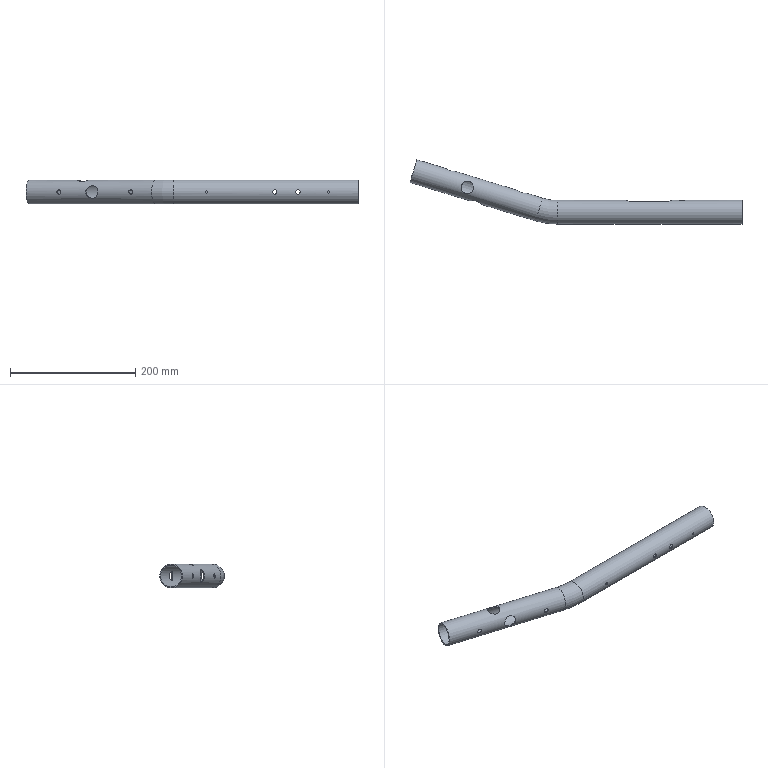Part | STEP file | PN_0042 | 1 solid | 23 faces | box 530.631 x 103.035 x 38.1 mm | volume 88372 mm3 | cylinder 17 | plane 4 | torus 2 | commonest cylinder face diameters 7 x4 3.5 x2 15 x2 18 x2 20 x2 35.1 x2